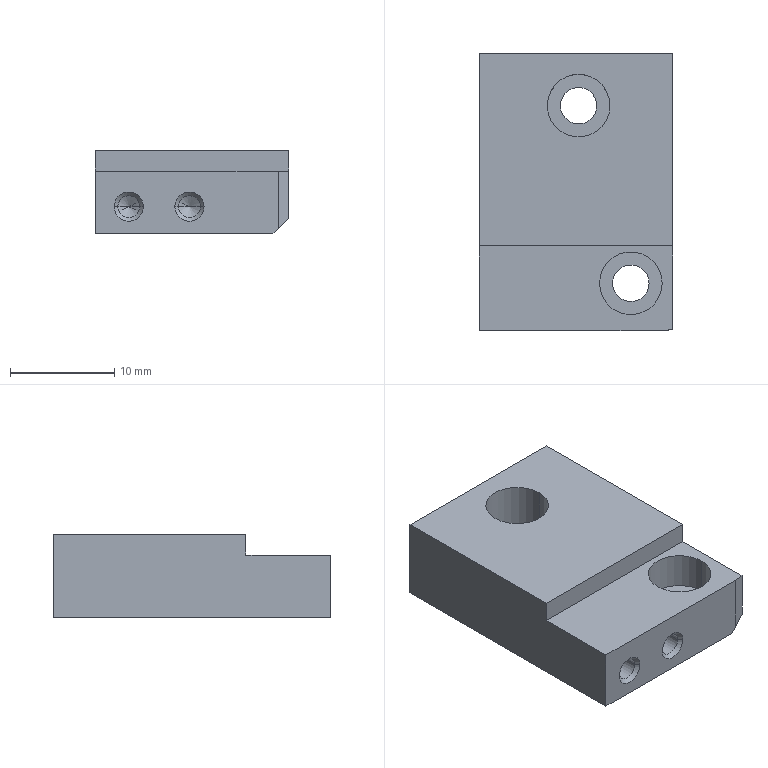Part | NX | 1 solid | 32 faces | box 18.5 x 26.53 x 8 mm | volume 3248 mm3 | plane 12 | cylinder 12 | cone 8 | commonest cylinder face diameters 2.1 x4 3.5 x4 6 x4
STEP:
#1=CARTESIAN_POINT('',(17.5,0.,6.));
#2=VERTEX_POINT('',#1);
#3=CARTESIAN_POINT('',(0.,0.,6.));
#4=VERTEX_POINT('',#3);
#5=CARTESIAN_POINT('',(0.,0.,6.));
#6=DIRECTION('',(-1.,0.,0.));
#7=VECTOR('',#6,1000.);
#8=LINE('',#5,#7);
#9=EDGE_CURVE('',#2,#4,#8,.T.);
#10=ORIENTED_EDGE('',*,*,#9,.T.);
#11=CARTESIAN_POINT('',(0.,0.,0.));
#12=VERTEX_POINT('',#11);
#13=CARTESIAN_POINT('',(0.,0.,0.));
#14=DIRECTION('',(0.,0.,1.));
#15=VECTOR('',#14,1000.);
#16=LINE('',#13,#15);
#17=EDGE_CURVE('',#12,#4,#16,.T.);
#18=ORIENTED_EDGE('',*,*,#17,.F.);
#19=CARTESIAN_POINT('',(17.,0.,0.));
#20=VERTEX_POINT('',#19);
#21=CARTESIAN_POINT('',(0.,0.,0.));
#22=DIRECTION('',(1.,0.,0.));
#23=VECTOR('',#22,1000.);
#24=LINE('',#21,#23);
#25=EDGE_CURVE('',#12,#20,#24,.T.);
#26=ORIENTED_EDGE('',*,*,#25,.T.);
#27=CARTESIAN_POINT('',(17.5,0.,0.5));
#28=VERTEX_POINT('',#27);
#29=CARTESIAN_POINT('',(17.,0.,0.));
#30=DIRECTION('',(-0.7071,0.,-0.7071));
#31=VECTOR('',#30,1000.);
#32=LINE('',#29,#31);
#33=EDGE_CURVE('',#28,#20,#32,.T.);
#34=ORIENTED_EDGE('',*,*,#33,.F.);
#35=CARTESIAN_POINT('',(17.5,0.,0.));
#36=DIRECTION('',(0.,0.,-1.));
#37=VECTOR('',#36,1000.);
#38=LINE('',#35,#37);
#39=EDGE_CURVE('',#2,#28,#38,.T.);
#40=ORIENTED_EDGE('',*,*,#39,.F.);
#41=EDGE_LOOP('',(#10,#18,#26,#34,#40));
#42=FACE_BOUND('',#41,.T.);
#43=CARTESIAN_POINT('',(10.4,0.,2.6));
#44=VERTEX_POINT('',#43);
#45=CARTESIAN_POINT('',(7.6,0.,2.6));
#46=VERTEX_POINT('',#45);
#47=CARTESIAN_POINT('',(9.,0.,2.6));
#48=DIRECTION('',(0.,-1.,0.));
#49=DIRECTION('',(-1.,0.,0.));
#50=AXIS2_PLACEMENT_3D('',#47,#48,#49);
#51=CIRCLE('',#50,1.4);
#52=EDGE_CURVE('',#44,#46,#51,.T.);
#53=ORIENTED_EDGE('',*,*,#52,.F.);
#54=CARTESIAN_POINT('',(9.,0.,2.6));
#55=DIRECTION('',(0.,-1.,0.));
#56=DIRECTION('',(-1.,0.,0.));
#57=AXIS2_PLACEMENT_3D('',#54,#55,#56);
#58=CIRCLE('',#57,1.4);
#59=EDGE_CURVE('',#46,#44,#58,.T.);
#60=ORIENTED_EDGE('',*,*,#59,.F.);
#61=EDGE_LOOP('',(#53,#60));
#62=FACE_BOUND('',#61,.T.);
#63=CARTESIAN_POINT('',(1.8,0.,2.6));
#64=VERTEX_POINT('',#63);
#65=CARTESIAN_POINT('',(4.6,0.,2.6));
#66=VERTEX_POINT('',#65);
#67=CARTESIAN_POINT('',(3.2,0.,2.6));
#68=DIRECTION('',(0.,-1.,0.));
#69=DIRECTION('',(-1.,0.,0.));
#70=AXIS2_PLACEMENT_3D('',#67,#68,#69);
#71=CIRCLE('',#70,1.4);
#72=EDGE_CURVE('',#64,#66,#71,.T.);
#73=ORIENTED_EDGE('',*,*,#72,.F.);
#74=CARTESIAN_POINT('',(3.2,0.,2.6));
#75=DIRECTION('',(0.,-1.,0.));
#76=DIRECTION('',(-1.,0.,0.));
#77=AXIS2_PLACEMENT_3D('',#74,#75,#76);
#78=CIRCLE('',#77,1.4);
#79=EDGE_CURVE('',#66,#64,#78,.T.);
#80=ORIENTED_EDGE('',*,*,#79,.F.);
#81=EDGE_LOOP('',(#73,#80));
#82=FACE_BOUND('',#81,.T.);
#83=CARTESIAN_POINT('',(0.,0.,0.));
#84=DIRECTION('',(0.,-1.,0.));
#85=DIRECTION('',(0.,0.,-1.));
#86=AXIS2_PLACEMENT_3D('',#83,#84,#85);
#87=PLANE('',#86);
#88=ADVANCED_FACE('',(#42,#62,#82),#87,.T.);
#89=CARTESIAN_POINT('',(18.5,8.1,8.));
#90=VERTEX_POINT('',#89);
#91=CARTESIAN_POINT('',(0.,8.1,8.));
#92=VERTEX_POINT('',#91);
#93=CARTESIAN_POINT('',(0.,8.1,8.));
#94=DIRECTION('',(-1.,0.,0.));
#95=VECTOR('',#94,1000.);
#96=LINE('',#93,#95);
#97=EDGE_CURVE('',#90,#92,#96,.T.);
#98=ORIENTED_EDGE('',*,*,#97,.F.);
#99=CARTESIAN_POINT('',(18.5,26.53,8.));
#100=VERTEX_POINT('',#99);
#101=CARTESIAN_POINT('',(18.5,0.,8.));
#102=DIRECTION('',(0.,1.,0.));
#103=VECTOR('',#102,1000.);
#104=LINE('',#101,#103);
#105=EDGE_CURVE('',#90,#100,#104,.T.);
#106=ORIENTED_EDGE('',*,*,#105,.T.);
#107=CARTESIAN_POINT('',(0.,26.53,8.));
#108=VERTEX_POINT('',#107);
#109=CARTESIAN_POINT('',(0.,26.53,8.));
#110=DIRECTION('',(1.,0.,0.));
#111=VECTOR('',#110,1000.);
#112=LINE('',#109,#111);
#113=EDGE_CURVE('',#108,#100,#112,.T.);
#114=ORIENTED_EDGE('',*,*,#113,.F.);
#115=CARTESIAN_POINT('',(0.,0.,8.));
#116=DIRECTION('',(0.,-1.,0.));
#117=VECTOR('',#116,1000.);
#118=LINE('',#115,#117);
#119=EDGE_CURVE('',#108,#92,#118,.T.);
#120=ORIENTED_EDGE('',*,*,#119,.T.);
#121=EDGE_LOOP('',(#98,#106,#114,#120));
#122=FACE_BOUND('',#121,.T.);
#123=CARTESIAN_POINT('',(12.5,21.53,8.));
#124=VERTEX_POINT('',#123);
#125=CARTESIAN_POINT('',(6.5,21.53,8.));
#126=VERTEX_POINT('',#125);
#127=CARTESIAN_POINT('',(9.5,21.53,8.));
#128=DIRECTION('',(0.,0.,1.));
#129=DIRECTION('',(1.,0.,0.));
#130=AXIS2_PLACEMENT_3D('',#127,#128,#129);
#131=CIRCLE('',#130,3.);
#132=EDGE_CURVE('',#124,#126,#131,.T.);
#133=ORIENTED_EDGE('',*,*,#132,.F.);
#134=CARTESIAN_POINT('',(9.5,21.53,8.));
#135=DIRECTION('',(0.,0.,1.));
#136=DIRECTION('',(1.,0.,0.));
#137=AXIS2_PLACEMENT_3D('',#134,#135,#136);
#138=CIRCLE('',#137,3.);
#139=EDGE_CURVE('',#126,#124,#138,.T.);
#140=ORIENTED_EDGE('',*,*,#139,.F.);
#141=EDGE_LOOP('',(#133,#140));
#142=FACE_BOUND('',#141,.T.);
#143=CARTESIAN_POINT('',(0.,0.,8.));
#144=DIRECTION('',(0.,0.,1.));
#145=DIRECTION('',(1.,0.,0.));
#146=AXIS2_PLACEMENT_3D('',#143,#144,#145);
#147=PLANE('',#146);
#148=ADVANCED_FACE('',(#122,#142),#147,.T.);
#149=ORIENTED_EDGE('',*,*,#9,.F.);
#150=CARTESIAN_POINT('',(18.5,0.08749,6.));
#151=VERTEX_POINT('',#150);
#152=CARTESIAN_POINT('',(0.,-1.531,6.));
#153=DIRECTION('',(0.9962,0.08716,0.));
#154=VECTOR('',#153,1000.);
#155=LINE('',#152,#154);
#156=EDGE_CURVE('',#2,#151,#155,.T.);
#157=ORIENTED_EDGE('',*,*,#156,.T.);
#158=CARTESIAN_POINT('',(18.5,8.1,6.));
#159=VERTEX_POINT('',#158);
#160=CARTESIAN_POINT('',(18.5,0.,6.));
#161=DIRECTION('',(0.,1.,0.));
#162=VECTOR('',#161,1000.);
#163=LINE('',#160,#162);
#164=EDGE_CURVE('',#151,#159,#163,.T.);
#165=ORIENTED_EDGE('',*,*,#164,.T.);
#166=CARTESIAN_POINT('',(0.,8.1,6.));
#167=VERTEX_POINT('',#166);
#168=CARTESIAN_POINT('',(0.,8.1,6.));
#169=DIRECTION('',(-1.,0.,0.));
#170=VECTOR('',#169,1000.);
#171=LINE('',#168,#170);
#172=EDGE_CURVE('',#159,#167,#171,.T.);
#173=ORIENTED_EDGE('',*,*,#172,.T.);
#174=CARTESIAN_POINT('',(0.,0.,6.));
#175=DIRECTION('',(0.,-1.,0.));
#176=VECTOR('',#175,1000.);
#177=LINE('',#174,#176);
#178=EDGE_CURVE('',#167,#4,#177,.T.);
#179=ORIENTED_EDGE('',*,*,#178,.T.);
#180=EDGE_LOOP('',(#149,#157,#165,#173,#179));
#181=FACE_BOUND('',#180,.T.);
#182=CARTESIAN_POINT('',(11.5,4.53,6.));
#183=VERTEX_POINT('',#182);
#184=CARTESIAN_POINT('',(17.5,4.53,6.));
#185=VERTEX_POINT('',#184);
#186=CARTESIAN_POINT('',(14.5,4.53,6.));
#187=DIRECTION('',(0.,0.,1.));
#188=DIRECTION('',(-1.,0.,0.));
#189=AXIS2_PLACEMENT_3D('',#186,#187,#188);
#190=CIRCLE('',#189,3.);
#191=EDGE_CURVE('',#183,#185,#190,.T.);
#192=ORIENTED_EDGE('',*,*,#191,.F.);
#193=CARTESIAN_POINT('',(14.5,4.53,6.));
#194=DIRECTION('',(0.,0.,1.));
#195=DIRECTION('',(-1.,0.,0.));
#196=AXIS2_PLACEMENT_3D('',#193,#194,#195);
#197=CIRCLE('',#196,3.);
#198=EDGE_CURVE('',#185,#183,#197,.T.);
#199=ORIENTED_EDGE('',*,*,#198,.F.);
#200=EDGE_LOOP('',(#192,#199));
#201=FACE_BOUND('',#200,.T.);
#202=CARTESIAN_POINT('',(18.5,0.,6.));
#203=DIRECTION('',(0.,0.,-1.));
#204=DIRECTION('',(0.,-1.,0.));
#205=AXIS2_PLACEMENT_3D('',#202,#203,#204);
#206=PLANE('',#205);
#207=ADVANCED_FACE('',(#181,#201),#206,.F.);
#208=ORIENTED_EDGE('',*,*,#178,.F.);
#209=CARTESIAN_POINT('',(0.,8.1,0.));
#210=DIRECTION('',(0.,0.,1.));
#211=VECTOR('',#210,1000.);
#212=LINE('',#209,#211);
#213=EDGE_CURVE('',#167,#92,#212,.T.);
#214=ORIENTED_EDGE('',*,*,#213,.T.);
#215=ORIENTED_EDGE('',*,*,#119,.F.);
#216=CARTESIAN_POINT('',(0.,26.53,0.));
#217=VERTEX_POINT('',#216);
#218=CARTESIAN_POINT('',(0.,26.53,0.));
#219=DIRECTION('',(0.,0.,1.));
#220=VECTOR('',#219,1000.);
#221=LINE('',#218,#220);
#222=EDGE_CURVE('',#217,#108,#221,.T.);
#223=ORIENTED_EDGE('',*,*,#222,.F.);
#224=CARTESIAN_POINT('',(0.,0.,0.));
#225=DIRECTION('',(0.,1.,0.));
#226=VECTOR('',#225,1000.);
#227=LINE('',#224,#226);
#228=EDGE_CURVE('',#12,#217,#227,.T.);
#229=ORIENTED_EDGE('',*,*,#228,.F.);
#230=ORIENTED_EDGE('',*,*,#17,.T.);
#231=EDGE_LOOP('',(#208,#214,#215,#223,#229,#230));
#232=FACE_BOUND('',#231,.T.);
#233=CARTESIAN_POINT('',(0.,26.53,0.));
#234=DIRECTION('',(-1.,0.,0.));
#235=DIRECTION('',(0.,0.,1.));
#236=AXIS2_PLACEMENT_3D('',#233,#234,#235);
#237=PLANE('',#236);
#238=ADVANCED_FACE('',(#232),#237,.T.);
#239=CARTESIAN_POINT('',(17.,26.53,0.));
#240=VERTEX_POINT('',#239);
#241=CARTESIAN_POINT('',(0.,26.53,0.));
#242=DIRECTION('',(1.,0.,0.));
#243=VECTOR('',#242,1000.);
#244=LINE('',#241,#243);
#245=EDGE_CURVE('',#217,#240,#244,.T.);
#246=ORIENTED_EDGE('',*,*,#245,.F.);
#247=ORIENTED_EDGE('',*,*,#222,.T.);
#248=ORIENTED_EDGE('',*,*,#113,.T.);
#249=CARTESIAN_POINT('',(18.5,26.53,1.5));
#250=VERTEX_POINT('',#249);
#251=CARTESIAN_POINT('',(18.5,26.53,0.));
#252=DIRECTION('',(0.,0.,-1.));
#253=VECTOR('',#252,1000.);
#254=LINE('',#251,#253);
#255=EDGE_CURVE('',#100,#250,#254,.T.);
#256=ORIENTED_EDGE('',*,*,#255,.T.);
#257=CARTESIAN_POINT('',(17.,26.53,0.));
#258=DIRECTION('',(0.7071,0.,0.7071));
#259=VECTOR('',#258,1000.);
#260=LINE('',#257,#259);
#261=EDGE_CURVE('',#240,#250,#260,.T.);
#262=ORIENTED_EDGE('',*,*,#261,.F.);
#263=EDGE_LOOP('',(#246,#247,#248,#256,#262));
#264=FACE_BOUND('',#263,.T.);
#265=CARTESIAN_POINT('',(18.5,26.53,0.));
#266=DIRECTION('',(0.,1.,0.));
#267=DIRECTION('',(1.,0.,0.));
#268=AXIS2_PLACEMENT_3D('',#265,#266,#267);
#269=PLANE('',#268);
#270=ADVANCED_FACE('',(#264),#269,.T.);
#271=CARTESIAN_POINT('',(17.,0.,0.));
#272=DIRECTION('',(0.,-1.,0.));
#273=VECTOR('',#272,1000.);
#274=LINE('',#271,#273);
#275=EDGE_CURVE('',#240,#20,#274,.T.);
#276=ORIENTED_EDGE('',*,*,#275,.F.);
#277=ORIENTED_EDGE('',*,*,#261,.T.);
#278=CARTESIAN_POINT('',(18.5,0.08749,1.5));
#279=VERTEX_POINT('',#278);
#280=CARTESIAN_POINT('',(18.5,0.,1.5));
#281=DIRECTION('',(0.,-1.,0.));
#282=VECTOR('',#281,1000.);
#283=LINE('',#280,#282);
#284=EDGE_CURVE('',#250,#279,#283,.T.);
#285=ORIENTED_EDGE('',*,*,#284,.T.);
#286=CARTESIAN_POINT('',(0.,-1.531,-17.));
#287=DIRECTION('',(-0.7058,-0.06175,-0.7058));
#288=VECTOR('',#287,1000.);
#289=LINE('',#286,#288);
#290=EDGE_CURVE('',#279,#28,#289,.T.);
#291=ORIENTED_EDGE('',*,*,#290,.T.);
#292=ORIENTED_EDGE('',*,*,#33,.T.);
#293=EDGE_LOOP('',(#276,#277,#285,#291,#292));
#294=FACE_BOUND('',#293,.T.);
#295=CARTESIAN_POINT('',(17.,0.,0.));
#296=DIRECTION('',(0.7071,0.,-0.7071));
#297=DIRECTION('',(0.,-1.,0.));
#298=AXIS2_PLACEMENT_3D('',#295,#296,#297);
#299=PLANE('',#298);
#300=ADVANCED_FACE('',(#294),#299,.T.);
#301=CARTESIAN_POINT('',(18.5,0.08749,0.));
#302=DIRECTION('',(0.,0.,1.));
#303=VECTOR('',#302,1000.);
#304=LINE('',#301,#303);
#305=EDGE_CURVE('',#279,#151,#304,.T.);
#306=ORIENTED_EDGE('',*,*,#305,.T.);
#307=ORIENTED_EDGE('',*,*,#156,.F.);
#308=ORIENTED_EDGE('',*,*,#39,.T.);
#309=ORIENTED_EDGE('',*,*,#290,.F.);
#310=EDGE_LOOP('',(#306,#307,#308,#309));
#311=FACE_BOUND('',#310,.T.);
#312=CARTESIAN_POINT('',(18.5,0.08749,1.5));
#313=DIRECTION('',(0.08716,-0.9962,0.));
#314=DIRECTION('',(0.,0.,-1.));
#315=AXIS2_PLACEMENT_3D('',#312,#313,#314);
#316=PLANE('',#315);
#317=ADVANCED_FACE('',(#311),#316,.T.);
#318=ORIENTED_EDGE('',*,*,#164,.F.);
#319=ORIENTED_EDGE('',*,*,#305,.F.);
#320=ORIENTED_EDGE('',*,*,#284,.F.);
#321=ORIENTED_EDGE('',*,*,#255,.F.);
#322=ORIENTED_EDGE('',*,*,#105,.F.);
#323=CARTESIAN_POINT('',(18.5,8.1,0.));
#324=DIRECTION('',(0.,0.,-1.));
#325=VECTOR('',#324,1000.);
#326=LINE('',#323,#325);
#327=EDGE_CURVE('',#90,#159,#326,.T.);
#328=ORIENTED_EDGE('',*,*,#327,.T.);
#329=EDGE_LOOP('',(#318,#319,#320,#321,#322,#328));
#330=FACE_BOUND('',#329,.T.);
#331=CARTESIAN_POINT('',(18.5,0.,0.));
#332=DIRECTION('',(1.,0.,0.));
#333=DIRECTION('',(0.,1.,0.));
#334=AXIS2_PLACEMENT_3D('',#331,#332,#333);
#335=PLANE('',#334);
#336=ADVANCED_FACE('',(#330),#335,.T.);
#337=ORIENTED_EDGE('',*,*,#97,.T.);
#338=ORIENTED_EDGE('',*,*,#213,.F.);
#339=ORIENTED_EDGE('',*,*,#172,.F.);
#340=ORIENTED_EDGE('',*,*,#327,.F.);
#341=EDGE_LOOP('',(#337,#338,#339,#340));
#342=FACE_BOUND('',#341,.T.);
#343=CARTESIAN_POINT('',(18.5,8.1,5.85));
#344=DIRECTION('',(0.,1.,0.));
#345=DIRECTION('',(1.,0.,0.));
#346=AXIS2_PLACEMENT_3D('',#343,#344,#345);
#347=PLANE('',#346);
#348=ADVANCED_FACE('',(#342),#347,.F.);
#349=ORIENTED_EDGE('',*,*,#25,.F.);
#350=ORIENTED_EDGE('',*,*,#228,.T.);
#351=ORIENTED_EDGE('',*,*,#245,.T.);
#352=ORIENTED_EDGE('',*,*,#275,.T.);
#353=EDGE_LOOP('',(#349,#350,#351,#352));
#354=FACE_BOUND('',#353,.T.);
#355=CARTESIAN_POINT('',(7.75,21.53,0.));
#356=VERTEX_POINT('',#355);
#357=CARTESIAN_POINT('',(11.25,21.53,0.));
#358=VERTEX_POINT('',#357);
#359=CARTESIAN_POINT('',(9.5,21.53,0.));
#360=DIRECTION('',(0.,0.,1.));
#361=DIRECTION('',(-1.,0.,0.));
#362=AXIS2_PLACEMENT_3D('',#359,#360,#361);
#363=CIRCLE('',#362,1.75);
#364=EDGE_CURVE('',#356,#358,#363,.T.);
#365=ORIENTED_EDGE('',*,*,#364,.T.);
#366=CARTESIAN_POINT('',(9.5,21.53,0.));
#367=DIRECTION('',(0.,0.,1.));
#368=DIRECTION('',(-1.,0.,0.));
#369=AXIS2_PLACEMENT_3D('',#366,#367,#368);
#370=CIRCLE('',#369,1.75);
#371=EDGE_CURVE('',#358,#356,#370,.T.);
#372=ORIENTED_EDGE('',*,*,#371,.T.);
#373=EDGE_LOOP('',(#365,#372));
#374=FACE_BOUND('',#373,.T.);
#375=CARTESIAN_POINT('',(12.75,4.53,0.));
#376=VERTEX_POINT('',#375);
#377=CARTESIAN_POINT('',(16.25,4.53,0.));
#378=VERTEX_POINT('',#377);
#379=CARTESIAN_POINT('',(14.5,4.53,0.));
#380=DIRECTION('',(0.,0.,1.));
#381=DIRECTION('',(-1.,0.,0.));
#382=AXIS2_PLACEMENT_3D('',#379,#380,#381);
#383=CIRCLE('',#382,1.75);
#384=EDGE_CURVE('',#376,#378,#383,.T.);
#385=ORIENTED_EDGE('',*,*,#384,.T.);
#386=CARTESIAN_POINT('',(14.5,4.53,0.));
#387=DIRECTION('',(0.,0.,1.));
#388=DIRECTION('',(-1.,0.,0.));
#389=AXIS2_PLACEMENT_3D('',#386,#387,#388);
#390=CIRCLE('',#389,1.75);
#391=EDGE_CURVE('',#378,#376,#390,.T.);
#392=ORIENTED_EDGE('',*,*,#391,.T.);
#393=EDGE_LOOP('',(#385,#392));
#394=FACE_BOUND('',#393,.T.);
#395=CARTESIAN_POINT('',(0.,0.,0.));
#396=DIRECTION('',(0.,0.,1.));
#397=DIRECTION('',(1.,0.,0.));
#398=AXIS2_PLACEMENT_3D('',#395,#396,#397);
#399=PLANE('',#398);
#400=ADVANCED_FACE('',(#354,#374,#394),#399,.F.);
#401=ORIENTED_EDGE('',*,*,#132,.T.);
#402=CARTESIAN_POINT('',(6.5,21.53,2.5));
#403=VERTEX_POINT('',#402);
#404=CARTESIAN_POINT('',(6.5,21.53,-1.24));
#405=DIRECTION('',(0.,0.,1.));
#406=VECTOR('',#405,1000.);
#407=LINE('',#404,#406);
#408=EDGE_CURVE('',#126,#403,#407,.F.);
#409=ORIENTED_EDGE('',*,*,#408,.T.);
#410=CARTESIAN_POINT('',(12.5,21.53,2.5));
#411=VERTEX_POINT('',#410);
#412=CARTESIAN_POINT('',(9.5,21.53,2.5));
#413=DIRECTION('',(0.,0.,-1.));
#414=DIRECTION('',(-1.,0.,0.));
#415=AXIS2_PLACEMENT_3D('',#412,#413,#414);
#416=CIRCLE('',#415,3.);
#417=EDGE_CURVE('',#403,#411,#416,.T.);
#418=ORIENTED_EDGE('',*,*,#417,.T.);
#419=CARTESIAN_POINT('',(12.5,21.53,-1.24));
#420=DIRECTION('',(0.,0.,1.));
#421=VECTOR('',#420,1000.);
#422=LINE('',#419,#421);
#423=EDGE_CURVE('',#124,#411,#422,.F.);
#424=ORIENTED_EDGE('',*,*,#423,.F.);
#425=EDGE_LOOP('',(#401,#409,#418,#424));
#426=FACE_BOUND('',#425,.T.);
#427=CARTESIAN_POINT('',(9.5,21.53,-1.24));
#428=DIRECTION('',(0.,0.,1.));
#429=DIRECTION('',(-1.,0.,0.));
#430=AXIS2_PLACEMENT_3D('',#427,#428,#429);
#431=CYLINDRICAL_SURFACE('',#430,3.);
#432=ADVANCED_FACE('',(#426),#431,.F.);
#433=CARTESIAN_POINT('',(7.95,6.3,2.6));
#434=VERTEX_POINT('',#433);
#435=CARTESIAN_POINT('',(10.05,6.3,2.6));
#436=VERTEX_POINT('',#435);
#437=CARTESIAN_POINT('',(9.,6.3,2.6));
#438=DIRECTION('',(0.,-1.,0.));
#439=DIRECTION('',(-1.,0.,0.));
#440=AXIS2_PLACEMENT_3D('',#437,#438,#439);
#441=CIRCLE('',#440,1.05);
#442=EDGE_CURVE('',#434,#436,#441,.T.);
#443=ORIENTED_EDGE('',*,*,#442,.T.);
#444=CARTESIAN_POINT('',(9.,6.931,2.6));
#445=VERTEX_POINT('',#444);
#446=CARTESIAN_POINT('',(9.542,6.605,2.6));
#447=DIRECTION('',(0.8572,-0.515,0.));
#448=VECTOR('',#447,1000.);
#449=LINE('',#446,#448);
#450=EDGE_CURVE('',#445,#436,#449,.T.);
#451=ORIENTED_EDGE('',*,*,#450,.F.);
#452=CARTESIAN_POINT('',(8.458,6.605,2.6));
#453=DIRECTION('',(-0.8572,-0.515,0.));
#454=VECTOR('',#453,1000.);
#455=LINE('',#452,#454);
#456=EDGE_CURVE('',#445,#434,#455,.T.);
#457=ORIENTED_EDGE('',*,*,#456,.T.);
#458=EDGE_LOOP('',(#443,#451,#457));
#459=FACE_BOUND('',#458,.T.);
#460=CARTESIAN_POINT('',(9.,6.605,2.6));
#461=DIRECTION('',(0.,-1.,0.));
#462=DIRECTION('',(-1.,0.,0.));
#463=AXIS2_PLACEMENT_3D('',#460,#461,#462);
#464=CONICAL_SURFACE('',#463,0.5421,1.03);
#465=ADVANCED_FACE('',(#459),#464,.F.);
#466=ORIENTED_EDGE('',*,*,#417,.F.);
#467=CARTESIAN_POINT('',(9.5,21.53,2.5));
#468=DIRECTION('',(0.,0.,-1.));
#469=DIRECTION('',(-1.,0.,0.));
#470=AXIS2_PLACEMENT_3D('',#467,#468,#469);
#471=CIRCLE('',#470,3.);
#472=EDGE_CURVE('',#411,#403,#471,.T.);
#473=ORIENTED_EDGE('',*,*,#472,.F.);
#474=EDGE_LOOP('',(#466,#473));
#475=FACE_BOUND('',#474,.T.);
#476=CARTESIAN_POINT('',(7.75,21.53,2.5));
#477=VERTEX_POINT('',#476);
#478=CARTESIAN_POINT('',(11.25,21.53,2.5));
#479=VERTEX_POINT('',#478);
#480=CARTESIAN_POINT('',(9.5,21.53,2.5));
#481=DIRECTION('',(0.,0.,1.));
#482=DIRECTION('',(-1.,0.,0.));
#483=AXIS2_PLACEMENT_3D('',#480,#481,#482);
#484=CIRCLE('',#483,1.75);
#485=EDGE_CURVE('',#477,#479,#484,.T.);
#486=ORIENTED_EDGE('',*,*,#485,.F.);
#487=CARTESIAN_POINT('',(9.5,21.53,2.5));
#488=DIRECTION('',(0.,0.,1.));
#489=DIRECTION('',(-1.,0.,0.));
#490=AXIS2_PLACEMENT_3D('',#487,#488,#489);
#491=CIRCLE('',#490,1.75);
#492=EDGE_CURVE('',#479,#477,#491,.T.);
#493=ORIENTED_EDGE('',*,*,#492,.F.);
#494=EDGE_LOOP('',(#486,#493));
#495=FACE_BOUND('',#494,.T.);
#496=CARTESIAN_POINT('',(9.5,21.53,2.5));
#497=DIRECTION('',(0.,0.,1.));
#498=DIRECTION('',(1.,0.,0.));
#499=AXIS2_PLACEMENT_3D('',#496,#497,#498);
#500=PLANE('',#499);
#501=ADVANCED_FACE('',(#475,#495),#500,.T.);
#502=ORIENTED_EDGE('',*,*,#485,.T.);
#503=CARTESIAN_POINT('',(11.25,21.53,-1.24));
#504=DIRECTION('',(0.,0.,1.));
#505=VECTOR('',#504,1000.);
#506=LINE('',#503,#505);
#507=EDGE_CURVE('',#479,#358,#506,.F.);
#508=ORIENTED_EDGE('',*,*,#507,.T.);
#509=ORIENTED_EDGE('',*,*,#364,.F.);
#510=CARTESIAN_POINT('',(7.75,21.53,-1.24));
#511=DIRECTION('',(0.,0.,1.));
#512=VECTOR('',#511,1000.);
#513=LINE('',#510,#512);
#514=EDGE_CURVE('',#477,#356,#513,.F.);
#515=ORIENTED_EDGE('',*,*,#514,.F.);
#516=EDGE_LOOP('',(#502,#508,#509,#515));
#517=FACE_BOUND('',#516,.T.);
#518=CARTESIAN_POINT('',(9.5,21.53,-1.24));
#519=DIRECTION('',(0.,0.,1.));
#520=DIRECTION('',(-1.,0.,0.));
#521=AXIS2_PLACEMENT_3D('',#518,#519,#520);
#522=CYLINDRICAL_SURFACE('',#521,1.75);
#523=ADVANCED_FACE('',(#517),#522,.F.);
#524=CARTESIAN_POINT('',(3.2,6.931,2.6));
#525=VERTEX_POINT('',#524);
#526=CARTESIAN_POINT('',(4.25,6.3,2.6));
#527=VERTEX_POINT('',#526);
#528=CARTESIAN_POINT('',(3.742,6.605,2.6));
#529=DIRECTION('',(0.8572,-0.515,0.));
#530=VECTOR('',#529,1000.);
#531=LINE('',#528,#530);
#532=EDGE_CURVE('',#525,#527,#531,.T.);
#533=ORIENTED_EDGE('',*,*,#532,.T.);
#534=CARTESIAN_POINT('',(2.15,6.3,2.6));
#535=VERTEX_POINT('',#534);
#536=CARTESIAN_POINT('',(3.2,6.3,2.6));
#537=DIRECTION('',(0.,-1.,0.));
#538=DIRECTION('',(-1.,0.,0.));
#539=AXIS2_PLACEMENT_3D('',#536,#537,#538);
#540=CIRCLE('',#539,1.05);
#541=EDGE_CURVE('',#527,#535,#540,.T.);
#542=ORIENTED_EDGE('',*,*,#541,.T.);
#543=CARTESIAN_POINT('',(2.658,6.605,2.6));
#544=DIRECTION('',(-0.8572,-0.515,0.));
#545=VECTOR('',#544,1000.);
#546=LINE('',#543,#545);
#547=EDGE_CURVE('',#525,#535,#546,.T.);
#548=ORIENTED_EDGE('',*,*,#547,.F.);
#549=EDGE_LOOP('',(#533,#542,#548));
#550=FACE_BOUND('',#549,.T.);
#551=CARTESIAN_POINT('',(3.2,6.605,2.6));
#552=DIRECTION('',(0.,-1.,0.));
#553=DIRECTION('',(-1.,0.,0.));
#554=AXIS2_PLACEMENT_3D('',#551,#552,#553);
#555=CONICAL_SURFACE('',#554,0.5421,1.03);
#556=ADVANCED_FACE('',(#550),#555,.F.);
#557=CARTESIAN_POINT('',(2.15,0.35,2.6));
#558=VERTEX_POINT('',#557);
#559=CARTESIAN_POINT('',(4.25,0.35,2.6));
#560=VERTEX_POINT('',#559);
#561=CARTESIAN_POINT('',(3.2,0.35,2.6));
#562=DIRECTION('',(0.,-1.,0.));
#563=DIRECTION('',(-1.,0.,0.));
#564=AXIS2_PLACEMENT_3D('',#561,#562,#563);
#565=CIRCLE('',#564,1.05);
#566=EDGE_CURVE('',#558,#560,#565,.T.);
#567=ORIENTED_EDGE('',*,*,#566,.T.);
#568=CARTESIAN_POINT('',(4.25,7.277,2.6));
#569=DIRECTION('',(0.,-1.,0.));
#570=VECTOR('',#569,1000.);
#571=LINE('',#568,#570);
#572=EDGE_CURVE('',#527,#560,#571,.T.);
#573=ORIENTED_EDGE('',*,*,#572,.F.);
#574=CARTESIAN_POINT('',(3.2,6.3,2.6));
#575=DIRECTION('',(0.,-1.,0.));
#576=DIRECTION('',(-1.,0.,0.));
#577=AXIS2_PLACEMENT_3D('',#574,#575,#576);
#578=CIRCLE('',#577,1.05);
#579=EDGE_CURVE('',#535,#527,#578,.T.);
#580=ORIENTED_EDGE('',*,*,#579,.F.);
#581=CARTESIAN_POINT('',(2.15,7.277,2.6));
#582=DIRECTION('',(0.,-1.,0.));
#583=VECTOR('',#582,1000.);
#584=LINE('',#581,#583);
#585=EDGE_CURVE('',#535,#558,#584,.T.);
#586=ORIENTED_EDGE('',*,*,#585,.T.);
#587=EDGE_LOOP('',(#567,#573,#580,#586));
#588=FACE_BOUND('',#587,.T.);
#589=CARTESIAN_POINT('',(3.2,7.277,2.6));
#590=DIRECTION('',(0.,-1.,0.));
#591=DIRECTION('',(-1.,0.,0.));
#592=AXIS2_PLACEMENT_3D('',#589,#590,#591);
#593=CYLINDRICAL_SURFACE('',#592,1.05);
#594=ADVANCED_FACE('',(#588),#593,.F.);
#595=ORIENTED_EDGE('',*,*,#442,.F.);
#596=CARTESIAN_POINT('',(7.95,0.35,2.6));
#597=VERTEX_POINT('',#596);
#598=CARTESIAN_POINT('',(7.95,7.277,2.6));
#599=DIRECTION('',(0.,-1.,0.));
#600=VECTOR('',#599,1000.);
#601=LINE('',#598,#600);
#602=EDGE_CURVE('',#597,#434,#601,.F.);
#603=ORIENTED_EDGE('',*,*,#602,.F.);
#604=CARTESIAN_POINT('',(10.05,0.35,2.6));
#605=VERTEX_POINT('',#604);
#606=CARTESIAN_POINT('',(9.,0.35,2.6));
#607=DIRECTION('',(0.,-1.,0.));
#608=DIRECTION('',(-1.,0.,0.));
#609=AXIS2_PLACEMENT_3D('',#606,#607,#608);
#610=CIRCLE('',#609,1.05);
#611=EDGE_CURVE('',#597,#605,#610,.T.);
#612=ORIENTED_EDGE('',*,*,#611,.T.);
#613=CARTESIAN_POINT('',(10.05,7.277,2.6));
#614=DIRECTION('',(0.,-1.,0.));
#615=VECTOR('',#614,1000.);
#616=LINE('',#613,#615);
#617=EDGE_CURVE('',#605,#436,#616,.F.);
#618=ORIENTED_EDGE('',*,*,#617,.T.);
#619=EDGE_LOOP('',(#595,#603,#612,#618));
#620=FACE_BOUND('',#619,.T.);
#621=CARTESIAN_POINT('',(9.,7.277,2.6));
#622=DIRECTION('',(0.,-1.,0.));
#623=DIRECTION('',(-1.,0.,0.));
#624=AXIS2_PLACEMENT_3D('',#621,#622,#623);
#625=CYLINDRICAL_SURFACE('',#624,1.05);
#626=ADVANCED_FACE('',(#620),#625,.F.);
#627=CARTESIAN_POINT('',(17.5,4.53,2.5));
#628=VERTEX_POINT('',#627);
#629=CARTESIAN_POINT('',(11.5,4.53,2.5));
#630=VERTEX_POINT('',#629);
#631=CARTESIAN_POINT('',(14.5,4.53,2.5));
#632=DIRECTION('',(0.,0.,1.));
#633=DIRECTION('',(-1.,0.,0.));
#634=AXIS2_PLACEMENT_3D('',#631,#632,#633);
#635=CIRCLE('',#634,3.);
#636=EDGE_CURVE('',#628,#630,#635,.T.);
#637=ORIENTED_EDGE('',*,*,#636,.F.);
#638=CARTESIAN_POINT('',(17.5,4.53,6.));
#639=DIRECTION('',(0.,0.,1.));
#640=VECTOR('',#639,1000.);
#641=LINE('',#638,#640);
#642=EDGE_CURVE('',#628,#185,#641,.T.);
#643=ORIENTED_EDGE('',*,*,#642,.T.);
#644=ORIENTED_EDGE('',*,*,#198,.T.);
#645=CARTESIAN_POINT('',(11.5,4.53,6.));
#646=DIRECTION('',(0.,0.,1.));
#647=VECTOR('',#646,1000.);
#648=LINE('',#645,#647);
#649=EDGE_CURVE('',#630,#183,#648,.T.);
#650=ORIENTED_EDGE('',*,*,#649,.F.);
#651=EDGE_LOOP('',(#637,#643,#644,#650));
#652=FACE_BOUND('',#651,.T.);
#653=CARTESIAN_POINT('',(14.5,4.53,6.));
#654=DIRECTION('',(0.,0.,1.));
#655=DIRECTION('',(-1.,0.,0.));
#656=AXIS2_PLACEMENT_3D('',#653,#654,#655);
#657=CYLINDRICAL_SURFACE('',#656,3.);
#658=ADVANCED_FACE('',(#652),#657,.F.);
#659=ORIENTED_EDGE('',*,*,#636,.T.);
#660=CARTESIAN_POINT('',(14.5,4.53,2.5));
#661=DIRECTION('',(0.,0.,1.));
#662=DIRECTION('',(-1.,0.,0.));
#663=AXIS2_PLACEMENT_3D('',#660,#661,#662);
#664=CIRCLE('',#663,3.);
#665=EDGE_CURVE('',#630,#628,#664,.T.);
#666=ORIENTED_EDGE('',*,*,#665,.T.);
#667=EDGE_LOOP('',(#659,#666));
#668=FACE_BOUND('',#667,.T.);
#669=CARTESIAN_POINT('',(16.25,4.53,2.5));
#670=VERTEX_POINT('',#669);
#671=CARTESIAN_POINT('',(12.75,4.53,2.5));
#672=VERTEX_POINT('',#671);
#673=CARTESIAN_POINT('',(14.5,4.53,2.5));
#674=DIRECTION('',(0.,0.,1.));
#675=DIRECTION('',(-1.,0.,0.));
#676=AXIS2_PLACEMENT_3D('',#673,#674,#675);
#677=CIRCLE('',#676,1.75);
#678=EDGE_CURVE('',#670,#672,#677,.T.);
#679=ORIENTED_EDGE('',*,*,#678,.F.);
#680=CARTESIAN_POINT('',(14.5,4.53,2.5));
#681=DIRECTION('',(0.,0.,1.));
#682=DIRECTION('',(-1.,0.,0.));
#683=AXIS2_PLACEMENT_3D('',#680,#681,#682);
#684=CIRCLE('',#683,1.75);
#685=EDGE_CURVE('',#672,#670,#684,.T.);
#686=ORIENTED_EDGE('',*,*,#685,.F.);
#687=EDGE_LOOP('',(#679,#686));
#688=FACE_BOUND('',#687,.T.);
#689=CARTESIAN_POINT('',(14.035,4.885,2.5));
#690=DIRECTION('',(0.,0.,1.));
#691=DIRECTION('',(1.,0.,0.));
#692=AXIS2_PLACEMENT_3D('',#689,#690,#691);
#693=PLANE('',#692);
#694=ADVANCED_FACE('',(#668,#688),#693,.T.);
#695=ORIENTED_EDGE('',*,*,#384,.F.);
#696=CARTESIAN_POINT('',(12.75,4.53,-0.8));
#697=DIRECTION('',(0.,0.,1.));
#698=VECTOR('',#697,1000.);
#699=LINE('',#696,#698);
#700=EDGE_CURVE('',#672,#376,#699,.F.);
#701=ORIENTED_EDGE('',*,*,#700,.F.);
#702=ORIENTED_EDGE('',*,*,#685,.T.);
#703=CARTESIAN_POINT('',(16.25,4.53,-0.8));
#704=DIRECTION('',(0.,0.,1.));
#705=VECTOR('',#704,1000.);
#706=LINE('',#703,#705);
#707=EDGE_CURVE('',#670,#378,#706,.F.);
#708=ORIENTED_EDGE('',*,*,#707,.T.);
#709=EDGE_LOOP('',(#695,#701,#702,#708));
#710=FACE_BOUND('',#709,.T.);
#711=CARTESIAN_POINT('',(14.5,4.53,-0.8));
#712=DIRECTION('',(0.,0.,1.));
#713=DIRECTION('',(-1.,0.,0.));
#714=AXIS2_PLACEMENT_3D('',#711,#712,#713);
#715=CYLINDRICAL_SURFACE('',#714,1.75);
#716=ADVANCED_FACE('',(#710),#715,.F.);
#717=ORIENTED_EDGE('',*,*,#72,.T.);
#718=CARTESIAN_POINT('',(4.6,0.,2.6));
#719=DIRECTION('',(0.7071,-0.7071,0.));
#720=VECTOR('',#719,1000.);
#721=LINE('',#718,#720);
#722=EDGE_CURVE('',#66,#560,#721,.F.);
#723=ORIENTED_EDGE('',*,*,#722,.T.);
#724=ORIENTED_EDGE('',*,*,#566,.F.);
#725=CARTESIAN_POINT('',(1.8,0.,2.6));
#726=DIRECTION('',(-0.7071,-0.7071,0.));
#727=VECTOR('',#726,1000.);
#728=LINE('',#725,#727);
#729=EDGE_CURVE('',#64,#558,#728,.F.);
#730=ORIENTED_EDGE('',*,*,#729,.F.);
#731=EDGE_LOOP('',(#717,#723,#724,#730));
#732=FACE_BOUND('',#731,.T.);
#733=CARTESIAN_POINT('',(3.2,0.,2.6));
#734=DIRECTION('',(0.,-1.,0.));
#735=DIRECTION('',(-1.,0.,0.));
#736=AXIS2_PLACEMENT_3D('',#733,#734,#735);
#737=CONICAL_SURFACE('',#736,1.4,0.7854);
#738=ADVANCED_FACE('',(#732),#737,.F.);
#739=ORIENTED_EDGE('',*,*,#611,.F.);
#740=CARTESIAN_POINT('',(7.6,0.,2.6));
#741=DIRECTION('',(-0.7071,-0.7071,0.));
#742=VECTOR('',#741,1000.);
#743=LINE('',#740,#742);
#744=EDGE_CURVE('',#46,#597,#743,.F.);
#745=ORIENTED_EDGE('',*,*,#744,.F.);
#746=ORIENTED_EDGE('',*,*,#59,.T.);
#747=CARTESIAN_POINT('',(10.4,0.,2.6));
#748=DIRECTION('',(0.7071,-0.7071,0.));
#749=VECTOR('',#748,1000.);
#750=LINE('',#747,#749);
#751=EDGE_CURVE('',#44,#605,#750,.F.);
#752=ORIENTED_EDGE('',*,*,#751,.T.);
#753=EDGE_LOOP('',(#739,#745,#746,#752));
#754=FACE_BOUND('',#753,.T.);
#755=CARTESIAN_POINT('',(9.,0.,2.6));
#756=DIRECTION('',(0.,-1.,0.));
#757=DIRECTION('',(-1.,0.,0.));
#758=AXIS2_PLACEMENT_3D('',#755,#756,#757);
#759=CONICAL_SURFACE('',#758,1.4,0.7854);
#760=ADVANCED_FACE('',(#754),#759,.F.);
#761=ORIENTED_EDGE('',*,*,#514,.T.);
#762=ORIENTED_EDGE('',*,*,#371,.F.);
#763=ORIENTED_EDGE('',*,*,#507,.F.);
#764=ORIENTED_EDGE('',*,*,#492,.T.);
#765=EDGE_LOOP('',(#761,#762,#763,#764));
#766=FACE_BOUND('',#765,.T.);
#767=CARTESIAN_POINT('',(9.5,21.53,-1.24));
#768=DIRECTION('',(0.,0.,1.));
#769=DIRECTION('',(-1.,0.,0.));
#770=AXIS2_PLACEMENT_3D('',#767,#768,#769);
#771=CYLINDRICAL_SURFACE('',#770,1.75);
#772=ADVANCED_FACE('',(#766),#771,.F.);
#773=ORIENTED_EDGE('',*,*,#729,.T.);
#774=CARTESIAN_POINT('',(3.2,0.35,2.6));
#775=DIRECTION('',(0.,-1.,0.));
#776=DIRECTION('',(-1.,0.,0.));
#777=AXIS2_PLACEMENT_3D('',#774,#775,#776);
#778=CIRCLE('',#777,1.05);
#779=EDGE_CURVE('',#560,#558,#778,.T.);
#780=ORIENTED_EDGE('',*,*,#779,.F.);
#781=ORIENTED_EDGE('',*,*,#722,.F.);
#782=ORIENTED_EDGE('',*,*,#79,.T.);
#783=EDGE_LOOP('',(#773,#780,#781,#782));
#784=FACE_BOUND('',#783,.T.);
#785=CARTESIAN_POINT('',(3.2,0.,2.6));
#786=DIRECTION('',(0.,-1.,0.));
#787=DIRECTION('',(-1.,0.,0.));
#788=AXIS2_PLACEMENT_3D('',#785,#786,#787);
#789=CONICAL_SURFACE('',#788,1.4,0.7854);
#790=ADVANCED_FACE('',(#784),#789,.F.);
#791=ORIENTED_EDGE('',*,*,#52,.T.);
#792=ORIENTED_EDGE('',*,*,#744,.T.);
#793=CARTESIAN_POINT('',(9.,0.35,2.6));
#794=DIRECTION('',(0.,-1.,0.));
#795=DIRECTION('',(-1.,0.,0.));
#796=AXIS2_PLACEMENT_3D('',#793,#794,#795);
#797=CIRCLE('',#796,1.05);
#798=EDGE_CURVE('',#605,#597,#797,.T.);
#799=ORIENTED_EDGE('',*,*,#798,.F.);
#800=ORIENTED_EDGE('',*,*,#751,.F.);
#801=EDGE_LOOP('',(#791,#792,#799,#800));
#802=FACE_BOUND('',#801,.T.);
#803=CARTESIAN_POINT('',(9.,0.,2.6));
#804=DIRECTION('',(0.,-1.,0.));
#805=DIRECTION('',(-1.,0.,0.));
#806=AXIS2_PLACEMENT_3D('',#803,#804,#805);
#807=CONICAL_SURFACE('',#806,1.4,0.7854);
#808=ADVANCED_FACE('',(#802),#807,.F.);
#809=ORIENTED_EDGE('',*,*,#408,.F.);
#810=ORIENTED_EDGE('',*,*,#139,.T.);
#811=ORIENTED_EDGE('',*,*,#423,.T.);
#812=ORIENTED_EDGE('',*,*,#472,.T.);
#813=EDGE_LOOP('',(#809,#810,#811,#812));
#814=FACE_BOUND('',#813,.T.);
#815=CARTESIAN_POINT('',(9.5,21.53,-1.24));
#816=DIRECTION('',(0.,0.,1.));
#817=DIRECTION('',(-1.,0.,0.));
#818=AXIS2_PLACEMENT_3D('',#815,#816,#817);
#819=CYLINDRICAL_SURFACE('',#818,3.);
#820=ADVANCED_FACE('',(#814),#819,.F.);
#821=ORIENTED_EDGE('',*,*,#678,.T.);
#822=ORIENTED_EDGE('',*,*,#700,.T.);
#823=ORIENTED_EDGE('',*,*,#391,.F.);
#824=ORIENTED_EDGE('',*,*,#707,.F.);
#825=EDGE_LOOP('',(#821,#822,#823,#824));
#826=FACE_BOUND('',#825,.T.);
#827=CARTESIAN_POINT('',(14.5,4.53,-0.8));
#828=DIRECTION('',(0.,0.,1.));
#829=DIRECTION('',(-1.,0.,0.));
#830=AXIS2_PLACEMENT_3D('',#827,#828,#829);
#831=CYLINDRICAL_SURFACE('',#830,1.75);
#832=ADVANCED_FACE('',(#826),#831,.F.);
#833=ORIENTED_EDGE('',*,*,#541,.F.);
#834=ORIENTED_EDGE('',*,*,#572,.T.);
#835=ORIENTED_EDGE('',*,*,#779,.T.);
#836=ORIENTED_EDGE('',*,*,#585,.F.);
#837=EDGE_LOOP('',(#833,#834,#835,#836));
#838=FACE_BOUND('',#837,.T.);
#839=CARTESIAN_POINT('',(3.2,7.277,2.6));
#840=DIRECTION('',(0.,-1.,0.));
#841=DIRECTION('',(-1.,0.,0.));
#842=AXIS2_PLACEMENT_3D('',#839,#840,#841);
#843=CYLINDRICAL_SURFACE('',#842,1.05);
#844=ADVANCED_FACE('',(#838),#843,.F.);
#845=ORIENTED_EDGE('',*,*,#602,.T.);
#846=CARTESIAN_POINT('',(9.,6.3,2.6));
#847=DIRECTION('',(0.,-1.,0.));
#848=DIRECTION('',(-1.,0.,0.));
#849=AXIS2_PLACEMENT_3D('',#846,#847,#848);
#850=CIRCLE('',#849,1.05);
#851=EDGE_CURVE('',#436,#434,#850,.T.);
#852=ORIENTED_EDGE('',*,*,#851,.F.);
#853=ORIENTED_EDGE('',*,*,#617,.F.);
#854=ORIENTED_EDGE('',*,*,#798,.T.);
#855=EDGE_LOOP('',(#845,#852,#853,#854));
#856=FACE_BOUND('',#855,.T.);
#857=CARTESIAN_POINT('',(9.,7.277,2.6));
#858=DIRECTION('',(0.,-1.,0.));
#859=DIRECTION('',(-1.,0.,0.));
#860=AXIS2_PLACEMENT_3D('',#857,#858,#859);
#861=CYLINDRICAL_SURFACE('',#860,1.05);
#862=ADVANCED_FACE('',(#856),#861,.F.);
#863=ORIENTED_EDGE('',*,*,#532,.F.);
#864=ORIENTED_EDGE('',*,*,#547,.T.);
#865=ORIENTED_EDGE('',*,*,#579,.T.);
#866=EDGE_LOOP('',(#863,#864,#865));
#867=FACE_BOUND('',#866,.T.);
#868=CARTESIAN_POINT('',(3.2,6.605,2.6));
#869=DIRECTION('',(0.,-1.,0.));
#870=DIRECTION('',(-1.,0.,0.));
#871=AXIS2_PLACEMENT_3D('',#868,#869,#870);
#872=CONICAL_SURFACE('',#871,0.5421,1.03);
#873=ADVANCED_FACE('',(#867),#872,.F.);
#874=ORIENTED_EDGE('',*,*,#191,.T.);
#875=ORIENTED_EDGE('',*,*,#642,.F.);
#876=ORIENTED_EDGE('',*,*,#665,.F.);
#877=ORIENTED_EDGE('',*,*,#649,.T.);
#878=EDGE_LOOP('',(#874,#875,#876,#877));
#879=FACE_BOUND('',#878,.T.);
#880=CARTESIAN_POINT('',(14.5,4.53,6.));
#881=DIRECTION('',(0.,0.,1.));
#882=DIRECTION('',(-1.,0.,0.));
#883=AXIS2_PLACEMENT_3D('',#880,#881,#882);
#884=CYLINDRICAL_SURFACE('',#883,3.);
#885=ADVANCED_FACE('',(#879),#884,.F.);
#886=ORIENTED_EDGE('',*,*,#450,.T.);
#887=ORIENTED_EDGE('',*,*,#851,.T.);
#888=ORIENTED_EDGE('',*,*,#456,.F.);
#889=EDGE_LOOP('',(#886,#887,#888));
#890=FACE_BOUND('',#889,.T.);
#891=CARTESIAN_POINT('',(9.,6.605,2.6));
#892=DIRECTION('',(0.,-1.,0.));
#893=DIRECTION('',(-1.,0.,0.));
#894=AXIS2_PLACEMENT_3D('',#891,#892,#893);
#895=CONICAL_SURFACE('',#894,0.5421,1.03);
#896=ADVANCED_FACE('',(#890),#895,.F.);
#897=CLOSED_SHELL('',(#88,#148,#207,#238,#270,#300,#317,#336,#348,#400,#432,#465,#501,#523,#556,#594,#626,#658,#694,#716,#738,#760,#772,#790,#808,#820,#832,#844,#862,#873,#885,#896));
#898=MANIFOLD_SOLID_BREP('',#897);
#899=(LENGTH_UNIT()NAMED_UNIT(*)SI_UNIT(.MILLI.,.METRE.));
#900=UNCERTAINTY_MEASURE_WITH_UNIT(LENGTH_MEASURE(0.00001),#899,'','');
#901=(NAMED_UNIT(*)PLANE_ANGLE_UNIT()SI_UNIT($,.RADIAN.));
#902=(NAMED_UNIT(*)SI_UNIT($,.STERADIAN.)SOLID_ANGLE_UNIT());
#903=(GEOMETRIC_REPRESENTATION_CONTEXT(3)GLOBAL_UNCERTAINTY_ASSIGNED_CONTEXT((#900))GLOBAL_UNIT_ASSIGNED_CONTEXT((#899,#901,#902))REPRESENTATION_CONTEXT('',''));
#904=ADVANCED_BREP_SHAPE_REPRESENTATION('',(#898),#903);